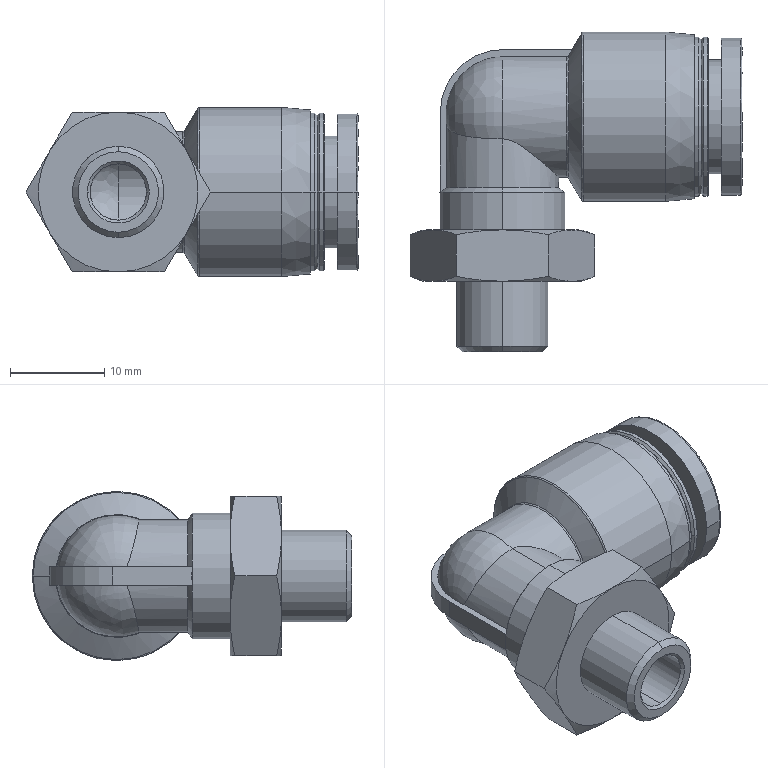Part | STEP file | Pipe fitting PL1001 | 1 solid | 89 faces | box 35.315 x 34 x 18 mm | volume 5648 mm3 | cylinder 28 | cone 28 | plane 19 | spline 12 | other 2 | commonest cylinder face diameters 8 x4 16.9 x4 12 x3 13.4 x3 6 x2 9.728 x2